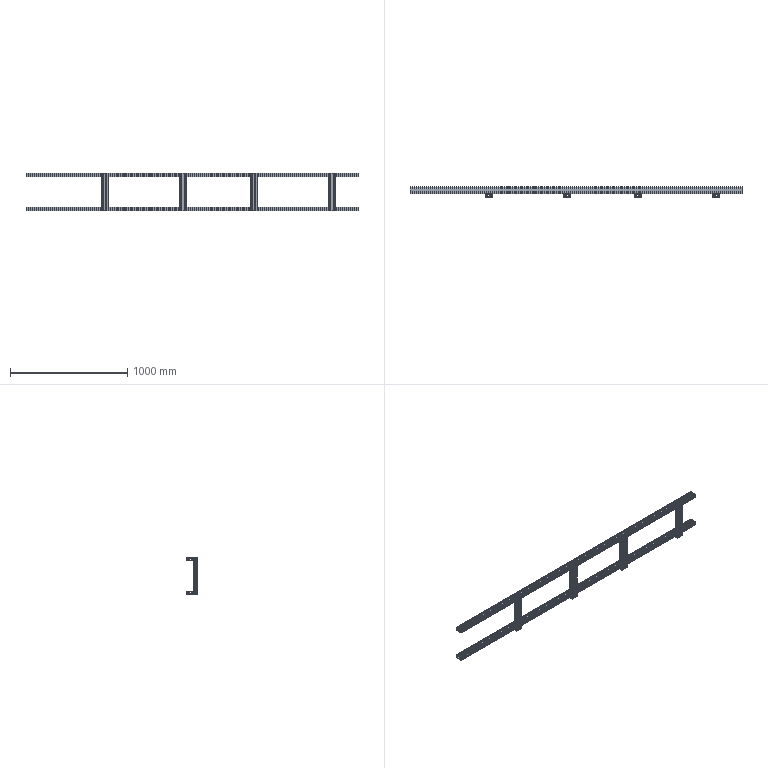Part | STEP file | Welding Conveyor Frame_Default<As Machined> | 6 solids | 700 faces | box 2830 x 90 x 316 mm | volume 3898026 mm3 | plane 564 | cylinder 136 | commonest cylinder face diameters 4.2 x48 0.6 x24 2 x24 8 x24 12 x16